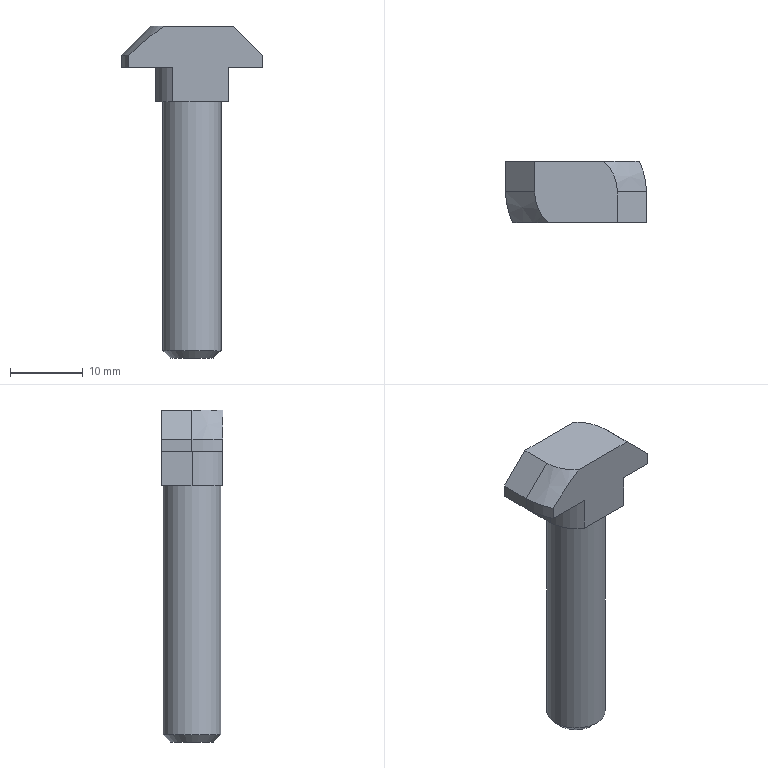Part | STEP file | 1_21 | 1 solid | 21 faces | box 19.4 x 8.5 x 45.7 mm | volume 2919 mm3 | plane 13 | cylinder 5 | cone 3 | commonest cylinder face diameters 10 x2 19.4 x2 8 x1